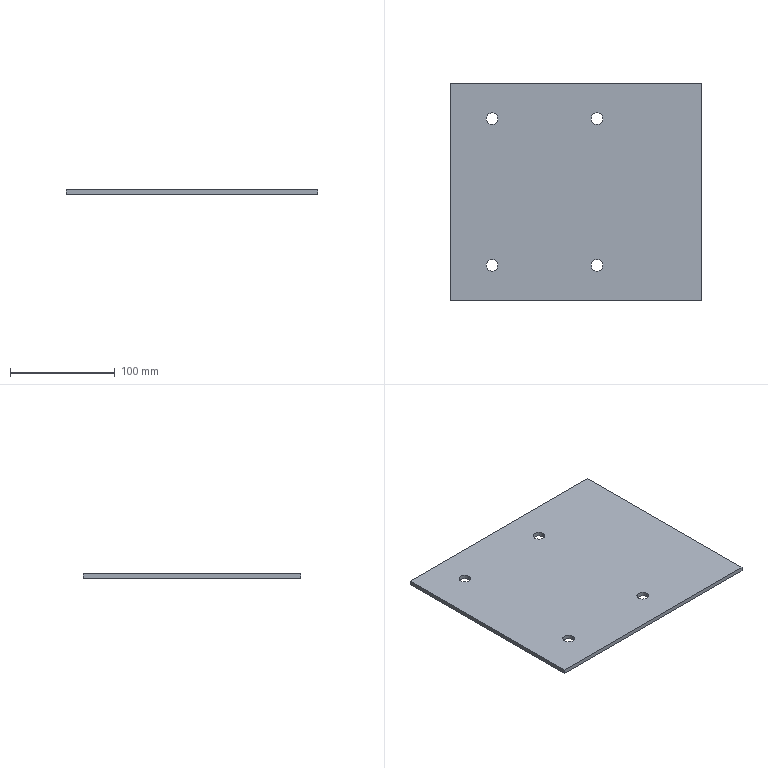Part | SolidWorks | features Cut 1, Extrusion 1 | 1 solid | 14 faces | box 240 x 208 x 4 mm | volume 198159 mm3 | cylinder 8 | plane 6 | commonest cylinder face diameters 11 x8
STEP:
#1=CARTESIAN_POINT('',(14.5,70.,4.));
#2=VERTEX_POINT('',#1);
#3=CARTESIAN_POINT('',(25.5,70.,4.));
#4=VERTEX_POINT('',#3);
#5=CARTESIAN_POINT('',(20.,70.,4.));
#6=DIRECTION('',(0.,0.,1.));
#7=DIRECTION('',(1.,0.,0.));
#8=AXIS2_PLACEMENT_3D('',#5,#6,#7);
#9=CIRCLE('',#8,5.5);
#10=EDGE_CURVE('',#2,#4,#9,.T.);
#11=ORIENTED_EDGE('',*,*,#10,.T.);
#12=CARTESIAN_POINT('',(25.5,70.,0.));
#13=VERTEX_POINT('',#12);
#14=CARTESIAN_POINT('',(25.5,70.,10.));
#15=DIRECTION('',(0.,0.,-1.));
#16=VECTOR('',#15,1000.);
#17=LINE('',#14,#16);
#18=EDGE_CURVE('',#4,#13,#17,.T.);
#19=ORIENTED_EDGE('',*,*,#18,.T.);
#20=CARTESIAN_POINT('',(14.5,70.,0.));
#21=VERTEX_POINT('',#20);
#22=CARTESIAN_POINT('',(20.,70.,0.));
#23=DIRECTION('',(0.,0.,-1.));
#24=DIRECTION('',(-1.,0.,0.));
#25=AXIS2_PLACEMENT_3D('',#22,#23,#24);
#26=CIRCLE('',#25,5.5);
#27=EDGE_CURVE('',#13,#21,#26,.T.);
#28=ORIENTED_EDGE('',*,*,#27,.T.);
#29=CARTESIAN_POINT('',(14.5,70.,10.));
#30=DIRECTION('',(0.,0.,-1.));
#31=VECTOR('',#30,1000.);
#32=LINE('',#29,#31);
#33=EDGE_CURVE('',#2,#21,#32,.T.);
#34=ORIENTED_EDGE('',*,*,#33,.F.);
#35=EDGE_LOOP('',(#11,#19,#28,#34));
#36=FACE_OUTER_BOUND('',#35,.T.);
#37=CARTESIAN_POINT('',(20.,70.,10.));
#38=DIRECTION('',(0.,0.,-1.));
#39=DIRECTION('',(-1.,0.,0.));
#40=AXIS2_PLACEMENT_3D('',#37,#38,#39);
#41=CYLINDRICAL_SURFACE('',#40,5.5);
#42=ADVANCED_FACE('',(#36),#41,.F.);
#43=CARTESIAN_POINT('',(-85.5,70.,4.));
#44=VERTEX_POINT('',#43);
#45=CARTESIAN_POINT('',(-74.5,70.,4.));
#46=VERTEX_POINT('',#45);
#47=CARTESIAN_POINT('',(-80.,70.,4.));
#48=DIRECTION('',(0.,0.,1.));
#49=DIRECTION('',(1.,0.,0.));
#50=AXIS2_PLACEMENT_3D('',#47,#48,#49);
#51=CIRCLE('',#50,5.5);
#52=EDGE_CURVE('',#44,#46,#51,.T.);
#53=ORIENTED_EDGE('',*,*,#52,.T.);
#54=CARTESIAN_POINT('',(-74.5,70.,0.));
#55=VERTEX_POINT('',#54);
#56=CARTESIAN_POINT('',(-74.5,70.,10.));
#57=DIRECTION('',(0.,0.,-1.));
#58=VECTOR('',#57,1000.);
#59=LINE('',#56,#58);
#60=EDGE_CURVE('',#46,#55,#59,.T.);
#61=ORIENTED_EDGE('',*,*,#60,.T.);
#62=CARTESIAN_POINT('',(-85.5,70.,0.));
#63=VERTEX_POINT('',#62);
#64=CARTESIAN_POINT('',(-80.,70.,0.));
#65=DIRECTION('',(0.,0.,-1.));
#66=DIRECTION('',(-1.,0.,0.));
#67=AXIS2_PLACEMENT_3D('',#64,#65,#66);
#68=CIRCLE('',#67,5.5);
#69=EDGE_CURVE('',#55,#63,#68,.T.);
#70=ORIENTED_EDGE('',*,*,#69,.T.);
#71=CARTESIAN_POINT('',(-85.5,70.,10.));
#72=DIRECTION('',(0.,0.,-1.));
#73=VECTOR('',#72,1000.);
#74=LINE('',#71,#73);
#75=EDGE_CURVE('',#44,#63,#74,.T.);
#76=ORIENTED_EDGE('',*,*,#75,.F.);
#77=EDGE_LOOP('',(#53,#61,#70,#76));
#78=FACE_OUTER_BOUND('',#77,.T.);
#79=CARTESIAN_POINT('',(-80.,70.,10.));
#80=DIRECTION('',(0.,0.,-1.));
#81=DIRECTION('',(-1.,0.,0.));
#82=AXIS2_PLACEMENT_3D('',#79,#80,#81);
#83=CYLINDRICAL_SURFACE('',#82,5.5);
#84=ADVANCED_FACE('',(#78),#83,.F.);
#85=CARTESIAN_POINT('',(-85.5,-70.,4.));
#86=VERTEX_POINT('',#85);
#87=CARTESIAN_POINT('',(-74.5,-70.,4.));
#88=VERTEX_POINT('',#87);
#89=CARTESIAN_POINT('',(-80.,-70.,4.));
#90=DIRECTION('',(0.,0.,1.));
#91=DIRECTION('',(1.,0.,0.));
#92=AXIS2_PLACEMENT_3D('',#89,#90,#91);
#93=CIRCLE('',#92,5.5);
#94=EDGE_CURVE('',#86,#88,#93,.T.);
#95=ORIENTED_EDGE('',*,*,#94,.T.);
#96=CARTESIAN_POINT('',(-74.5,-70.,0.));
#97=VERTEX_POINT('',#96);
#98=CARTESIAN_POINT('',(-74.5,-70.,10.));
#99=DIRECTION('',(0.,0.,-1.));
#100=VECTOR('',#99,1000.);
#101=LINE('',#98,#100);
#102=EDGE_CURVE('',#88,#97,#101,.T.);
#103=ORIENTED_EDGE('',*,*,#102,.T.);
#104=CARTESIAN_POINT('',(-85.5,-70.,0.));
#105=VERTEX_POINT('',#104);
#106=CARTESIAN_POINT('',(-80.,-70.,0.));
#107=DIRECTION('',(0.,0.,-1.));
#108=DIRECTION('',(-1.,0.,0.));
#109=AXIS2_PLACEMENT_3D('',#106,#107,#108);
#110=CIRCLE('',#109,5.5);
#111=EDGE_CURVE('',#97,#105,#110,.T.);
#112=ORIENTED_EDGE('',*,*,#111,.T.);
#113=CARTESIAN_POINT('',(-85.5,-70.,10.));
#114=DIRECTION('',(0.,0.,-1.));
#115=VECTOR('',#114,1000.);
#116=LINE('',#113,#115);
#117=EDGE_CURVE('',#86,#105,#116,.T.);
#118=ORIENTED_EDGE('',*,*,#117,.F.);
#119=EDGE_LOOP('',(#95,#103,#112,#118));
#120=FACE_OUTER_BOUND('',#119,.T.);
#121=CARTESIAN_POINT('',(-80.,-70.,10.));
#122=DIRECTION('',(0.,0.,-1.));
#123=DIRECTION('',(-1.,0.,0.));
#124=AXIS2_PLACEMENT_3D('',#121,#122,#123);
#125=CYLINDRICAL_SURFACE('',#124,5.5);
#126=ADVANCED_FACE('',(#120),#125,.F.);
#127=CARTESIAN_POINT('',(14.5,-70.,4.));
#128=VERTEX_POINT('',#127);
#129=CARTESIAN_POINT('',(25.5,-70.,4.));
#130=VERTEX_POINT('',#129);
#131=CARTESIAN_POINT('',(20.,-70.,4.));
#132=DIRECTION('',(0.,0.,1.));
#133=DIRECTION('',(1.,0.,0.));
#134=AXIS2_PLACEMENT_3D('',#131,#132,#133);
#135=CIRCLE('',#134,5.5);
#136=EDGE_CURVE('',#128,#130,#135,.T.);
#137=ORIENTED_EDGE('',*,*,#136,.T.);
#138=CARTESIAN_POINT('',(25.5,-70.,0.));
#139=VERTEX_POINT('',#138);
#140=CARTESIAN_POINT('',(25.5,-70.,10.));
#141=DIRECTION('',(0.,0.,-1.));
#142=VECTOR('',#141,1000.);
#143=LINE('',#140,#142);
#144=EDGE_CURVE('',#130,#139,#143,.T.);
#145=ORIENTED_EDGE('',*,*,#144,.T.);
#146=CARTESIAN_POINT('',(14.5,-70.,0.));
#147=VERTEX_POINT('',#146);
#148=CARTESIAN_POINT('',(20.,-70.,0.));
#149=DIRECTION('',(0.,0.,-1.));
#150=DIRECTION('',(-1.,0.,0.));
#151=AXIS2_PLACEMENT_3D('',#148,#149,#150);
#152=CIRCLE('',#151,5.5);
#153=EDGE_CURVE('',#139,#147,#152,.T.);
#154=ORIENTED_EDGE('',*,*,#153,.T.);
#155=CARTESIAN_POINT('',(14.5,-70.,10.));
#156=DIRECTION('',(0.,0.,-1.));
#157=VECTOR('',#156,1000.);
#158=LINE('',#155,#157);
#159=EDGE_CURVE('',#128,#147,#158,.T.);
#160=ORIENTED_EDGE('',*,*,#159,.F.);
#161=EDGE_LOOP('',(#137,#145,#154,#160));
#162=FACE_OUTER_BOUND('',#161,.T.);
#163=CARTESIAN_POINT('',(20.,-70.,10.));
#164=DIRECTION('',(0.,0.,-1.));
#165=DIRECTION('',(-1.,0.,0.));
#166=AXIS2_PLACEMENT_3D('',#163,#164,#165);
#167=CYLINDRICAL_SURFACE('',#166,5.5);
#168=ADVANCED_FACE('',(#162),#167,.F.);
#169=CARTESIAN_POINT('',(-120.,104.,0.));
#170=VERTEX_POINT('',#169);
#171=CARTESIAN_POINT('',(-120.,-104.,0.));
#172=VERTEX_POINT('',#171);
#173=CARTESIAN_POINT('',(-120.,-104.,0.));
#174=DIRECTION('',(0.,-1.,0.));
#175=VECTOR('',#174,1000.);
#176=LINE('',#173,#175);
#177=EDGE_CURVE('',#170,#172,#176,.T.);
#178=ORIENTED_EDGE('',*,*,#177,.T.);
#179=CARTESIAN_POINT('',(-120.,-104.,4.));
#180=VERTEX_POINT('',#179);
#181=CARTESIAN_POINT('',(-120.,-104.,4.));
#182=DIRECTION('',(0.,0.,-1.));
#183=VECTOR('',#182,1000.);
#184=LINE('',#181,#183);
#185=EDGE_CURVE('',#180,#172,#184,.T.);
#186=ORIENTED_EDGE('',*,*,#185,.F.);
#187=CARTESIAN_POINT('',(-120.,104.,4.));
#188=VERTEX_POINT('',#187);
#189=CARTESIAN_POINT('',(-120.,-104.,4.));
#190=DIRECTION('',(0.,-1.,0.));
#191=VECTOR('',#190,1000.);
#192=LINE('',#189,#191);
#193=EDGE_CURVE('',#188,#180,#192,.T.);
#194=ORIENTED_EDGE('',*,*,#193,.F.);
#195=CARTESIAN_POINT('',(-120.,104.,4.));
#196=DIRECTION('',(0.,0.,-1.));
#197=VECTOR('',#196,1000.);
#198=LINE('',#195,#197);
#199=EDGE_CURVE('',#188,#170,#198,.T.);
#200=ORIENTED_EDGE('',*,*,#199,.T.);
#201=EDGE_LOOP('',(#178,#186,#194,#200));
#202=FACE_OUTER_BOUND('',#201,.T.);
#203=CARTESIAN_POINT('',(-120.,-104.,4.));
#204=DIRECTION('',(1.,0.,0.));
#205=DIRECTION('',(0.,0.,-1.));
#206=AXIS2_PLACEMENT_3D('',#203,#204,#205);
#207=PLANE('',#206);
#208=ADVANCED_FACE('',(#202),#207,.F.);
#209=CARTESIAN_POINT('',(120.,-104.,0.));
#210=VERTEX_POINT('',#209);
#211=CARTESIAN_POINT('',(120.,-104.,0.));
#212=DIRECTION('',(1.,0.,0.));
#213=VECTOR('',#212,1000.);
#214=LINE('',#211,#213);
#215=EDGE_CURVE('',#172,#210,#214,.T.);
#216=ORIENTED_EDGE('',*,*,#215,.T.);
#217=CARTESIAN_POINT('',(120.,-104.,4.));
#218=VERTEX_POINT('',#217);
#219=CARTESIAN_POINT('',(120.,-104.,4.));
#220=DIRECTION('',(0.,0.,-1.));
#221=VECTOR('',#220,1000.);
#222=LINE('',#219,#221);
#223=EDGE_CURVE('',#218,#210,#222,.T.);
#224=ORIENTED_EDGE('',*,*,#223,.F.);
#225=CARTESIAN_POINT('',(120.,-104.,4.));
#226=DIRECTION('',(1.,0.,0.));
#227=VECTOR('',#226,1000.);
#228=LINE('',#225,#227);
#229=EDGE_CURVE('',#180,#218,#228,.T.);
#230=ORIENTED_EDGE('',*,*,#229,.F.);
#231=ORIENTED_EDGE('',*,*,#185,.T.);
#232=EDGE_LOOP('',(#216,#224,#230,#231));
#233=FACE_OUTER_BOUND('',#232,.T.);
#234=CARTESIAN_POINT('',(120.,-104.,4.));
#235=DIRECTION('',(0.,1.,0.));
#236=DIRECTION('',(-1.,0.,0.));
#237=AXIS2_PLACEMENT_3D('',#234,#235,#236);
#238=PLANE('',#237);
#239=ADVANCED_FACE('',(#233),#238,.F.);
#240=CARTESIAN_POINT('',(120.,104.,0.));
#241=VERTEX_POINT('',#240);
#242=CARTESIAN_POINT('',(120.,-104.,0.));
#243=DIRECTION('',(0.,1.,0.));
#244=VECTOR('',#243,1000.);
#245=LINE('',#242,#244);
#246=EDGE_CURVE('',#210,#241,#245,.T.);
#247=ORIENTED_EDGE('',*,*,#246,.T.);
#248=CARTESIAN_POINT('',(120.,104.,4.));
#249=VERTEX_POINT('',#248);
#250=CARTESIAN_POINT('',(120.,104.,4.));
#251=DIRECTION('',(0.,0.,-1.));
#252=VECTOR('',#251,1000.);
#253=LINE('',#250,#252);
#254=EDGE_CURVE('',#249,#241,#253,.T.);
#255=ORIENTED_EDGE('',*,*,#254,.F.);
#256=CARTESIAN_POINT('',(120.,-104.,4.));
#257=DIRECTION('',(0.,1.,0.));
#258=VECTOR('',#257,1000.);
#259=LINE('',#256,#258);
#260=EDGE_CURVE('',#218,#249,#259,.T.);
#261=ORIENTED_EDGE('',*,*,#260,.F.);
#262=ORIENTED_EDGE('',*,*,#223,.T.);
#263=EDGE_LOOP('',(#247,#255,#261,#262));
#264=FACE_OUTER_BOUND('',#263,.T.);
#265=CARTESIAN_POINT('',(120.,-104.,4.));
#266=DIRECTION('',(-1.,0.,0.));
#267=DIRECTION('',(0.,0.,1.));
#268=AXIS2_PLACEMENT_3D('',#265,#266,#267);
#269=PLANE('',#268);
#270=ADVANCED_FACE('',(#264),#269,.F.);
#271=CARTESIAN_POINT('',(120.,104.,0.));
#272=DIRECTION('',(-1.,0.,0.));
#273=VECTOR('',#272,1000.);
#274=LINE('',#271,#273);
#275=EDGE_CURVE('',#241,#170,#274,.T.);
#276=ORIENTED_EDGE('',*,*,#275,.T.);
#277=ORIENTED_EDGE('',*,*,#199,.F.);
#278=CARTESIAN_POINT('',(120.,104.,4.));
#279=DIRECTION('',(-1.,0.,0.));
#280=VECTOR('',#279,1000.);
#281=LINE('',#278,#280);
#282=EDGE_CURVE('',#249,#188,#281,.T.);
#283=ORIENTED_EDGE('',*,*,#282,.F.);
#284=ORIENTED_EDGE('',*,*,#254,.T.);
#285=EDGE_LOOP('',(#276,#277,#283,#284));
#286=FACE_OUTER_BOUND('',#285,.T.);
#287=CARTESIAN_POINT('',(120.,104.,4.));
#288=DIRECTION('',(0.,-1.,0.));
#289=DIRECTION('',(1.,0.,0.));
#290=AXIS2_PLACEMENT_3D('',#287,#288,#289);
#291=PLANE('',#290);
#292=ADVANCED_FACE('',(#286),#291,.F.);
#293=ORIENTED_EDGE('',*,*,#10,.F.);
#294=CARTESIAN_POINT('',(20.,70.,4.));
#295=DIRECTION('',(0.,0.,1.));
#296=DIRECTION('',(1.,0.,0.));
#297=AXIS2_PLACEMENT_3D('',#294,#295,#296);
#298=CIRCLE('',#297,5.5);
#299=EDGE_CURVE('',#4,#2,#298,.T.);
#300=ORIENTED_EDGE('',*,*,#299,.F.);
#301=EDGE_LOOP('',(#293,#300));
#302=FACE_BOUND('',#301,.T.);
#303=ORIENTED_EDGE('',*,*,#52,.F.);
#304=CARTESIAN_POINT('',(-80.,70.,4.));
#305=DIRECTION('',(0.,0.,1.));
#306=DIRECTION('',(1.,0.,0.));
#307=AXIS2_PLACEMENT_3D('',#304,#305,#306);
#308=CIRCLE('',#307,5.5);
#309=EDGE_CURVE('',#46,#44,#308,.T.);
#310=ORIENTED_EDGE('',*,*,#309,.F.);
#311=EDGE_LOOP('',(#303,#310));
#312=FACE_BOUND('',#311,.T.);
#313=ORIENTED_EDGE('',*,*,#94,.F.);
#314=CARTESIAN_POINT('',(-80.,-70.,4.));
#315=DIRECTION('',(0.,0.,1.));
#316=DIRECTION('',(1.,0.,0.));
#317=AXIS2_PLACEMENT_3D('',#314,#315,#316);
#318=CIRCLE('',#317,5.5);
#319=EDGE_CURVE('',#88,#86,#318,.T.);
#320=ORIENTED_EDGE('',*,*,#319,.F.);
#321=EDGE_LOOP('',(#313,#320));
#322=FACE_BOUND('',#321,.T.);
#323=ORIENTED_EDGE('',*,*,#136,.F.);
#324=CARTESIAN_POINT('',(20.,-70.,4.));
#325=DIRECTION('',(0.,0.,1.));
#326=DIRECTION('',(1.,0.,0.));
#327=AXIS2_PLACEMENT_3D('',#324,#325,#326);
#328=CIRCLE('',#327,5.5);
#329=EDGE_CURVE('',#130,#128,#328,.T.);
#330=ORIENTED_EDGE('',*,*,#329,.F.);
#331=EDGE_LOOP('',(#323,#330));
#332=FACE_BOUND('',#331,.T.);
#333=ORIENTED_EDGE('',*,*,#193,.T.);
#334=ORIENTED_EDGE('',*,*,#229,.T.);
#335=ORIENTED_EDGE('',*,*,#260,.T.);
#336=ORIENTED_EDGE('',*,*,#282,.T.);
#337=EDGE_LOOP('',(#333,#334,#335,#336));
#338=FACE_OUTER_BOUND('',#337,.T.);
#339=CARTESIAN_POINT('',(0.,0.,4.));
#340=DIRECTION('',(0.,0.,1.));
#341=DIRECTION('',(1.,0.,0.));
#342=AXIS2_PLACEMENT_3D('',#339,#340,#341);
#343=PLANE('',#342);
#344=ADVANCED_FACE('',(#302,#312,#322,#332,#338),#343,.T.);
#345=CARTESIAN_POINT('',(20.,70.,0.));
#346=DIRECTION('',(0.,0.,-1.));
#347=DIRECTION('',(-1.,0.,0.));
#348=AXIS2_PLACEMENT_3D('',#345,#346,#347);
#349=CIRCLE('',#348,5.5);
#350=EDGE_CURVE('',#21,#13,#349,.T.);
#351=ORIENTED_EDGE('',*,*,#350,.F.);
#352=ORIENTED_EDGE('',*,*,#27,.F.);
#353=EDGE_LOOP('',(#351,#352));
#354=FACE_BOUND('',#353,.T.);
#355=CARTESIAN_POINT('',(-80.,70.,0.));
#356=DIRECTION('',(0.,0.,-1.));
#357=DIRECTION('',(-1.,0.,0.));
#358=AXIS2_PLACEMENT_3D('',#355,#356,#357);
#359=CIRCLE('',#358,5.5);
#360=EDGE_CURVE('',#63,#55,#359,.T.);
#361=ORIENTED_EDGE('',*,*,#360,.F.);
#362=ORIENTED_EDGE('',*,*,#69,.F.);
#363=EDGE_LOOP('',(#361,#362));
#364=FACE_BOUND('',#363,.T.);
#365=CARTESIAN_POINT('',(-80.,-70.,0.));
#366=DIRECTION('',(0.,0.,-1.));
#367=DIRECTION('',(-1.,0.,0.));
#368=AXIS2_PLACEMENT_3D('',#365,#366,#367);
#369=CIRCLE('',#368,5.5);
#370=EDGE_CURVE('',#105,#97,#369,.T.);
#371=ORIENTED_EDGE('',*,*,#370,.F.);
#372=ORIENTED_EDGE('',*,*,#111,.F.);
#373=EDGE_LOOP('',(#371,#372));
#374=FACE_BOUND('',#373,.T.);
#375=CARTESIAN_POINT('',(20.,-70.,0.));
#376=DIRECTION('',(0.,0.,-1.));
#377=DIRECTION('',(-1.,0.,0.));
#378=AXIS2_PLACEMENT_3D('',#375,#376,#377);
#379=CIRCLE('',#378,5.5);
#380=EDGE_CURVE('',#147,#139,#379,.T.);
#381=ORIENTED_EDGE('',*,*,#380,.F.);
#382=ORIENTED_EDGE('',*,*,#153,.F.);
#383=EDGE_LOOP('',(#381,#382));
#384=FACE_BOUND('',#383,.T.);
#385=ORIENTED_EDGE('',*,*,#177,.F.);
#386=ORIENTED_EDGE('',*,*,#275,.F.);
#387=ORIENTED_EDGE('',*,*,#246,.F.);
#388=ORIENTED_EDGE('',*,*,#215,.F.);
#389=EDGE_LOOP('',(#385,#386,#387,#388));
#390=FACE_OUTER_BOUND('',#389,.T.);
#391=CARTESIAN_POINT('',(0.,0.,0.));
#392=DIRECTION('',(0.,0.,1.));
#393=DIRECTION('',(1.,0.,0.));
#394=AXIS2_PLACEMENT_3D('',#391,#392,#393);
#395=PLANE('',#394);
#396=ADVANCED_FACE('',(#354,#364,#374,#384,#390),#395,.F.);
#397=ORIENTED_EDGE('',*,*,#144,.F.);
#398=ORIENTED_EDGE('',*,*,#329,.T.);
#399=ORIENTED_EDGE('',*,*,#159,.T.);
#400=ORIENTED_EDGE('',*,*,#380,.T.);
#401=EDGE_LOOP('',(#397,#398,#399,#400));
#402=FACE_OUTER_BOUND('',#401,.T.);
#403=CARTESIAN_POINT('',(20.,-70.,10.));
#404=DIRECTION('',(0.,0.,-1.));
#405=DIRECTION('',(-1.,0.,0.));
#406=AXIS2_PLACEMENT_3D('',#403,#404,#405);
#407=CYLINDRICAL_SURFACE('',#406,5.5);
#408=ADVANCED_FACE('',(#402),#407,.F.);
#409=ORIENTED_EDGE('',*,*,#102,.F.);
#410=ORIENTED_EDGE('',*,*,#319,.T.);
#411=ORIENTED_EDGE('',*,*,#117,.T.);
#412=ORIENTED_EDGE('',*,*,#370,.T.);
#413=EDGE_LOOP('',(#409,#410,#411,#412));
#414=FACE_OUTER_BOUND('',#413,.T.);
#415=CARTESIAN_POINT('',(-80.,-70.,10.));
#416=DIRECTION('',(0.,0.,-1.));
#417=DIRECTION('',(-1.,0.,0.));
#418=AXIS2_PLACEMENT_3D('',#415,#416,#417);
#419=CYLINDRICAL_SURFACE('',#418,5.5);
#420=ADVANCED_FACE('',(#414),#419,.F.);
#421=ORIENTED_EDGE('',*,*,#60,.F.);
#422=ORIENTED_EDGE('',*,*,#309,.T.);
#423=ORIENTED_EDGE('',*,*,#75,.T.);
#424=ORIENTED_EDGE('',*,*,#360,.T.);
#425=EDGE_LOOP('',(#421,#422,#423,#424));
#426=FACE_OUTER_BOUND('',#425,.T.);
#427=CARTESIAN_POINT('',(-80.,70.,10.));
#428=DIRECTION('',(0.,0.,-1.));
#429=DIRECTION('',(-1.,0.,0.));
#430=AXIS2_PLACEMENT_3D('',#427,#428,#429);
#431=CYLINDRICAL_SURFACE('',#430,5.5);
#432=ADVANCED_FACE('',(#426),#431,.F.);
#433=ORIENTED_EDGE('',*,*,#18,.F.);
#434=ORIENTED_EDGE('',*,*,#299,.T.);
#435=ORIENTED_EDGE('',*,*,#33,.T.);
#436=ORIENTED_EDGE('',*,*,#350,.T.);
#437=EDGE_LOOP('',(#433,#434,#435,#436));
#438=FACE_OUTER_BOUND('',#437,.T.);
#439=CARTESIAN_POINT('',(20.,70.,10.));
#440=DIRECTION('',(0.,0.,-1.));
#441=DIRECTION('',(-1.,0.,0.));
#442=AXIS2_PLACEMENT_3D('',#439,#440,#441);
#443=CYLINDRICAL_SURFACE('',#442,5.5);
#444=ADVANCED_FACE('',(#438),#443,.F.);
#445=CLOSED_SHELL('',(#42,#84,#126,#168,#208,#239,#270,#292,#344,#396,#408,#420,#432,#444));
#446=MANIFOLD_SOLID_BREP('',#445);
#447=CARTESIAN_POINT('',(0.,0.,0.));
#448=DIRECTION('',(0.,0.,1.));
#449=DIRECTION('',(1.,0.,0.));
#450=AXIS2_PLACEMENT_3D('',#447,#448,#449);
#451=(LENGTH_UNIT()NAMED_UNIT(*)SI_UNIT(.MILLI.,.METRE.));
#452=UNCERTAINTY_MEASURE_WITH_UNIT(LENGTH_MEASURE(0.00001),#451,'','');
#453=(NAMED_UNIT(*)PLANE_ANGLE_UNIT()SI_UNIT($,.RADIAN.));
#454=(NAMED_UNIT(*)SI_UNIT($,.STERADIAN.)SOLID_ANGLE_UNIT());
#455=(GEOMETRIC_REPRESENTATION_CONTEXT(3)GLOBAL_UNCERTAINTY_ASSIGNED_CONTEXT((#452))GLOBAL_UNIT_ASSIGNED_CONTEXT((#451,#453,#454))REPRESENTATION_CONTEXT('',''));
#456=ADVANCED_BREP_SHAPE_REPRESENTATION('',(#446,#450),#455);